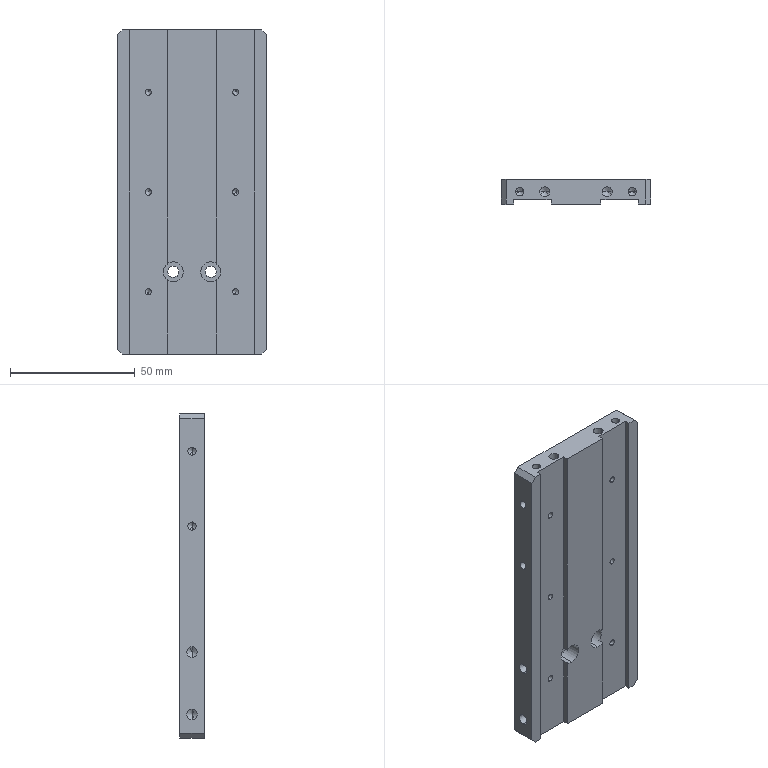Part | STEP file | PN_0021 | 1 solid | 102 faces | box 60 x 10 x 130 mm | volume 67558 mm3 | cylinder 44 | cone 36 | plane 22 | commonest cylinder face diameters 2.5 x12 3.3 x12 4.2 x8 4 x4 4.5 x4 8 x4